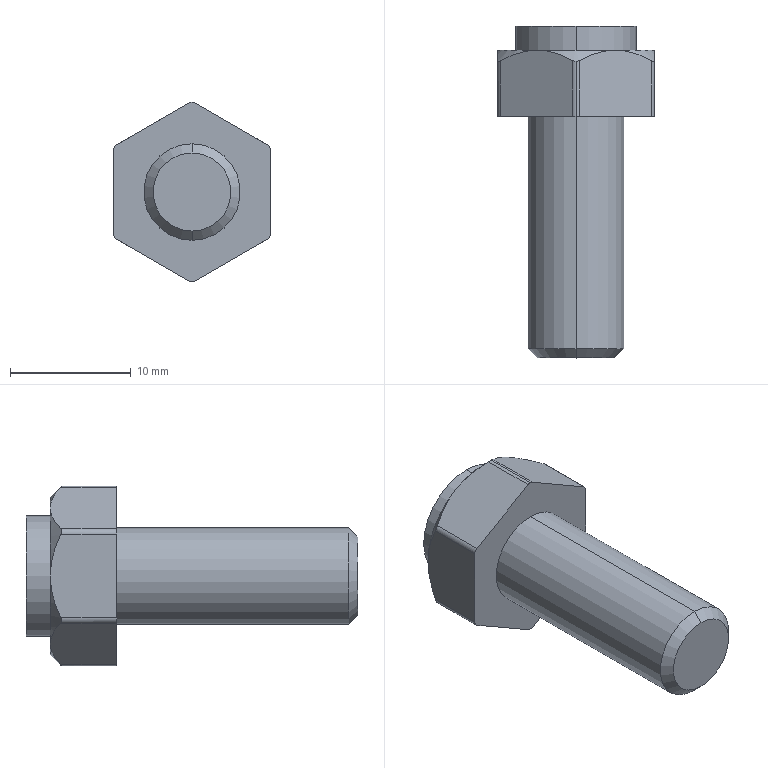Part | STEP file | TDB71-M8-L20-001^TDB71-M8-L20_Cylinder clamp assembly | 1 solid | 30 faces | box 13 x 27.5 x 14.856 mm | volume 1956 mm3 | cylinder 11 | plane 10 | cone 9 | commonest cylinder face diameters 1 x7 8 x2 10 x2